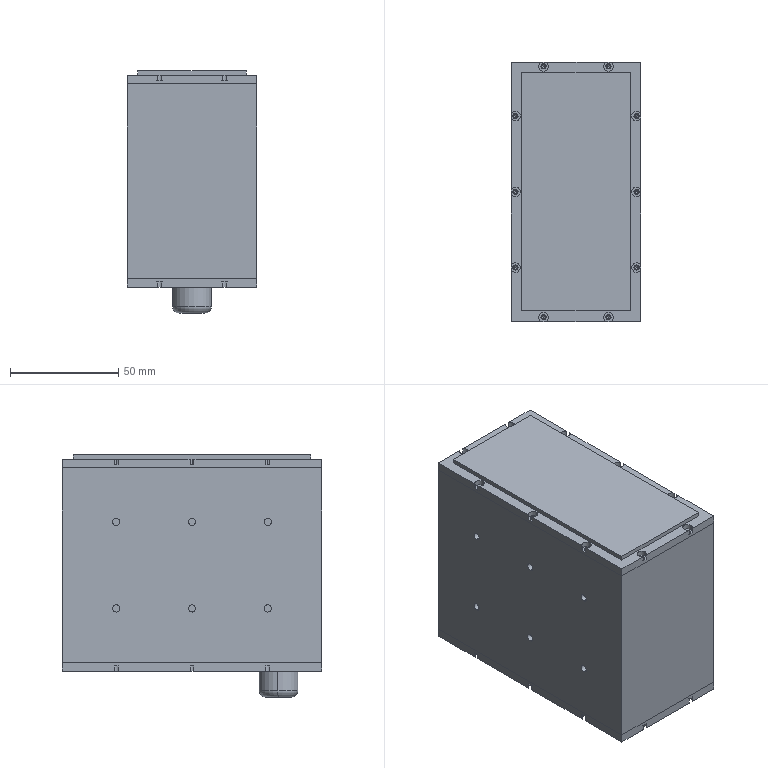Part | SolidWorks | features InContextFeatHolder 4 | 12 solids | 336 faces | box 60 x 120 x 112 mm | volume 205676 mm3 | cylinder 194 | plane 90 | cone 48 | torus 4 | commonest cylinder face diameters 4.4 x42 1.6 x40 2.4 x40 3.3 x24 2.5 x16 3.4 x8